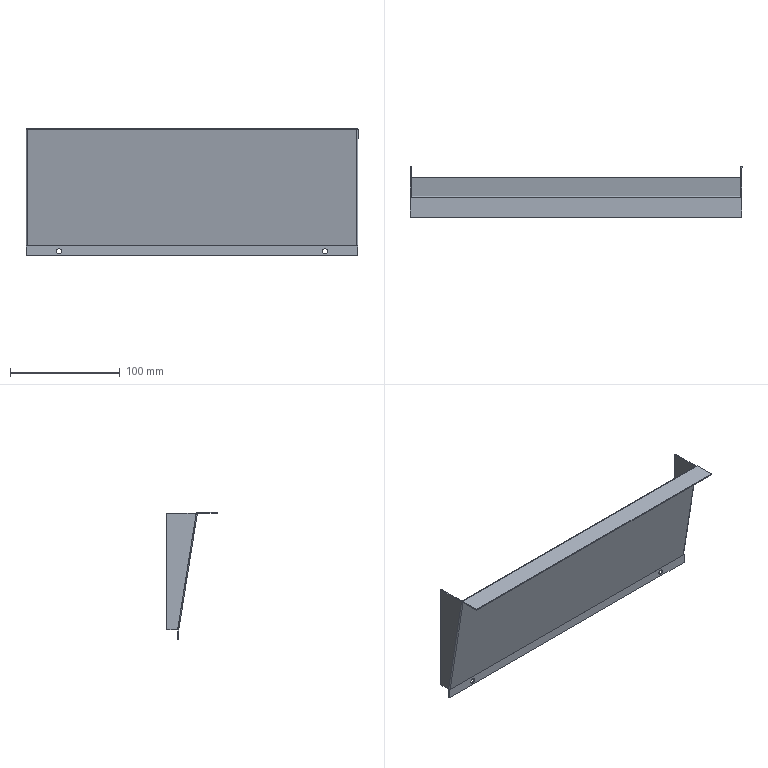Part | SolidWorks | features Cut 1, EdgeFlange 1, FlatPattern 1, MirrorPattern 1, SMBaseFlange 1, SheetMetal 1, UnFold 1 | 1 solid | 46 faces | box 302 x 46 x 116 mm | volume 44658 mm3 | plane 30 | cylinder 12 | spline 4 | commonest cylinder face diameters 0.2 x4 2.2 x4 4.5 x4
STEP:
#1=CARTESIAN_POINT('',(121.,-1.,-2.75));
#2=VERTEX_POINT('',#1);
#3=CARTESIAN_POINT('',(121.,-1.,-7.25));
#4=VERTEX_POINT('',#3);
#5=CARTESIAN_POINT('',(121.,-1.,-5.));
#6=DIRECTION('',(0.,-1.,0.));
#7=DIRECTION('',(0.,0.,-1.));
#8=AXIS2_PLACEMENT_3D('',#5,#6,#7);
#9=CIRCLE('',#8,2.25);
#10=EDGE_CURVE('',#2,#4,#9,.T.);
#11=ORIENTED_EDGE('',*,*,#10,.T.);
#12=CARTESIAN_POINT('',(121.,0.,-7.25));
#13=VERTEX_POINT('',#12);
#14=CARTESIAN_POINT('',(121.,-10.,-7.25));
#15=DIRECTION('',(0.,1.,0.));
#16=VECTOR('',#15,1000.);
#17=LINE('',#14,#16);
#18=EDGE_CURVE('',#4,#13,#17,.T.);
#19=ORIENTED_EDGE('',*,*,#18,.T.);
#20=CARTESIAN_POINT('',(121.,0.,-2.75));
#21=VERTEX_POINT('',#20);
#22=CARTESIAN_POINT('',(121.,0.,-5.));
#23=DIRECTION('',(0.,1.,0.));
#24=DIRECTION('',(0.,0.,1.));
#25=AXIS2_PLACEMENT_3D('',#22,#23,#24);
#26=CIRCLE('',#25,2.25);
#27=EDGE_CURVE('',#13,#21,#26,.T.);
#28=ORIENTED_EDGE('',*,*,#27,.T.);
#29=CARTESIAN_POINT('',(121.,-10.,-2.75));
#30=DIRECTION('',(0.,1.,0.));
#31=VECTOR('',#30,1000.);
#32=LINE('',#29,#31);
#33=EDGE_CURVE('',#2,#21,#32,.T.);
#34=ORIENTED_EDGE('',*,*,#33,.F.);
#35=EDGE_LOOP('',(#11,#19,#28,#34));
#36=FACE_OUTER_BOUND('',#35,.T.);
#37=CARTESIAN_POINT('',(121.,-10.,-5.));
#38=DIRECTION('',(0.,1.,0.));
#39=DIRECTION('',(0.,0.,1.));
#40=AXIS2_PLACEMENT_3D('',#37,#38,#39);
#41=CYLINDRICAL_SURFACE('',#40,2.25);
#42=ADVANCED_FACE('',(#36),#41,.F.);
#43=CARTESIAN_POINT('',(-121.,-1.,-2.75));
#44=VERTEX_POINT('',#43);
#45=CARTESIAN_POINT('',(-121.,-1.,-7.25));
#46=VERTEX_POINT('',#45);
#47=CARTESIAN_POINT('',(-121.,-1.,-5.));
#48=DIRECTION('',(0.,-1.,0.));
#49=DIRECTION('',(0.,0.,-1.));
#50=AXIS2_PLACEMENT_3D('',#47,#48,#49);
#51=CIRCLE('',#50,2.25);
#52=EDGE_CURVE('',#44,#46,#51,.T.);
#53=ORIENTED_EDGE('',*,*,#52,.T.);
#54=CARTESIAN_POINT('',(-121.,0.,-7.25));
#55=VERTEX_POINT('',#54);
#56=CARTESIAN_POINT('',(-121.,-10.,-7.25));
#57=DIRECTION('',(0.,1.,0.));
#58=VECTOR('',#57,1000.);
#59=LINE('',#56,#58);
#60=EDGE_CURVE('',#46,#55,#59,.T.);
#61=ORIENTED_EDGE('',*,*,#60,.T.);
#62=CARTESIAN_POINT('',(-121.,0.,-2.75));
#63=VERTEX_POINT('',#62);
#64=CARTESIAN_POINT('',(-121.,0.,-5.));
#65=DIRECTION('',(0.,1.,0.));
#66=DIRECTION('',(0.,0.,-1.));
#67=AXIS2_PLACEMENT_3D('',#64,#65,#66);
#68=CIRCLE('',#67,2.25);
#69=EDGE_CURVE('',#55,#63,#68,.T.);
#70=ORIENTED_EDGE('',*,*,#69,.T.);
#71=CARTESIAN_POINT('',(-121.,-10.,-2.75));
#72=DIRECTION('',(0.,1.,0.));
#73=VECTOR('',#72,1000.);
#74=LINE('',#71,#73);
#75=EDGE_CURVE('',#44,#63,#74,.T.);
#76=ORIENTED_EDGE('',*,*,#75,.F.);
#77=EDGE_LOOP('',(#53,#61,#70,#76));
#78=FACE_OUTER_BOUND('',#77,.T.);
#79=CARTESIAN_POINT('',(-121.,-10.,-5.));
#80=DIRECTION('',(0.,1.,0.));
#81=DIRECTION('',(0.,0.,1.));
#82=AXIS2_PLACEMENT_3D('',#79,#80,#81);
#83=CYLINDRICAL_SURFACE('',#82,2.25);
#84=ADVANCED_FACE('',(#78),#83,.F.);
#85=CARTESIAN_POINT('',(-149.9,-17.939,106.));
#86=VERTEX_POINT('',#85);
#87=CARTESIAN_POINT('',(-149.9,-17.939,107.));
#88=VERTEX_POINT('',#87);
#89=CARTESIAN_POINT('',(-149.9,-17.939,106.));
#90=DIRECTION('',(0.,0.,1.));
#91=VECTOR('',#90,1000.);
#92=LINE('',#89,#91);
#93=EDGE_CURVE('',#86,#88,#92,.T.);
#94=ORIENTED_EDGE('',*,*,#93,.F.);
#95=CARTESIAN_POINT('',(-151.,-17.939,106.));
#96=VERTEX_POINT('',#95);
#97=CARTESIAN_POINT('',(151.,-17.939,106.));
#98=DIRECTION('',(-1.,0.,0.));
#99=VECTOR('',#98,1000.);
#100=LINE('',#97,#99);
#101=EDGE_CURVE('',#86,#96,#100,.T.);
#102=ORIENTED_EDGE('',*,*,#101,.T.);
#103=CARTESIAN_POINT('',(-151.,-17.939,107.));
#104=VERTEX_POINT('',#103);
#105=CARTESIAN_POINT('',(-151.,-17.939,107.));
#106=DIRECTION('',(0.,0.,-1.));
#107=VECTOR('',#106,1000.);
#108=LINE('',#105,#107);
#109=EDGE_CURVE('',#104,#96,#108,.T.);
#110=ORIENTED_EDGE('',*,*,#109,.F.);
#111=CARTESIAN_POINT('',(151.,-17.939,107.));
#112=DIRECTION('',(-1.,0.,0.));
#113=VECTOR('',#112,1000.);
#114=LINE('',#111,#113);
#115=EDGE_CURVE('',#88,#104,#114,.T.);
#116=ORIENTED_EDGE('',*,*,#115,.F.);
#117=EDGE_LOOP('',(#94,#102,#110,#116));
#118=FACE_OUTER_BOUND('',#117,.T.);
#119=CARTESIAN_POINT('',(0.,-17.939,0.));
#120=DIRECTION('',(0.,-1.,0.));
#121=DIRECTION('',(0.,0.,-1.));
#122=AXIS2_PLACEMENT_3D('',#119,#120,#121);
#123=PLANE('',#122);
#124=ADVANCED_FACE('',(#118),#123,.F.);
#125=CARTESIAN_POINT('',(149.9,-17.939,106.));
#126=VERTEX_POINT('',#125);
#127=CARTESIAN_POINT('',(151.,-17.939,106.));
#128=DIRECTION('',(-1.,0.,0.));
#129=VECTOR('',#128,1000.);
#130=LINE('',#127,#129);
#131=EDGE_CURVE('',#126,#86,#130,.T.);
#132=ORIENTED_EDGE('',*,*,#131,.T.);
#133=CARTESIAN_POINT('',(-149.9,-17.84,105.916));
#134=VERTEX_POINT('',#133);
#135=CARTESIAN_POINT('',(-149.9,-17.939,105.9));
#136=DIRECTION('',(-1.,0.,0.));
#137=DIRECTION('',(0.,0.,1.));
#138=AXIS2_PLACEMENT_3D('',#135,#136,#137);
#139=CIRCLE('',#138,0.1);
#140=EDGE_CURVE('',#86,#134,#139,.T.);
#141=ORIENTED_EDGE('',*,*,#140,.T.);
#142=CARTESIAN_POINT('',(149.9,-17.84,105.916));
#143=VERTEX_POINT('',#142);
#144=CARTESIAN_POINT('',(151.,-17.84,105.916));
#145=DIRECTION('',(-1.,0.,0.));
#146=VECTOR('',#145,1000.);
#147=LINE('',#144,#146);
#148=EDGE_CURVE('',#143,#134,#147,.T.);
#149=ORIENTED_EDGE('',*,*,#148,.F.);
#150=CARTESIAN_POINT('',(149.9,-17.939,105.9));
#151=DIRECTION('',(1.,0.,0.));
#152=DIRECTION('',(0.,0.,-1.));
#153=AXIS2_PLACEMENT_3D('',#150,#151,#152);
#154=CIRCLE('',#153,0.1);
#155=EDGE_CURVE('',#143,#126,#154,.T.);
#156=ORIENTED_EDGE('',*,*,#155,.T.);
#157=EDGE_LOOP('',(#132,#141,#149,#156));
#158=FACE_OUTER_BOUND('',#157,.T.);
#159=CARTESIAN_POINT('',(151.,-17.939,105.9));
#160=DIRECTION('',(-1.,0.,0.));
#161=DIRECTION('',(0.,0.,1.));
#162=AXIS2_PLACEMENT_3D('',#159,#160,#161);
#163=CYLINDRICAL_SURFACE('',#162,0.1);
#164=ADVANCED_FACE('',(#158),#163,.F.);
#165=CARTESIAN_POINT('',(-149.9,0.,-0.08684));
#166=VERTEX_POINT('',#165);
#167=CARTESIAN_POINT('',(-149.9,-1.,-0.08684));
#168=VERTEX_POINT('',#167);
#169=CARTESIAN_POINT('',(-149.9,0.,-0.08684));
#170=DIRECTION('',(0.,-1.,0.));
#171=VECTOR('',#170,1000.);
#172=LINE('',#169,#171);
#173=EDGE_CURVE('',#166,#168,#172,.T.);
#174=ORIENTED_EDGE('',*,*,#173,.F.);
#175=CARTESIAN_POINT('',(-151.,0.,-0.08684));
#176=VERTEX_POINT('',#175);
#177=CARTESIAN_POINT('',(151.,0.,-0.08684));
#178=DIRECTION('',(-1.,0.,0.));
#179=VECTOR('',#178,1000.);
#180=LINE('',#177,#179);
#181=EDGE_CURVE('',#166,#176,#180,.T.);
#182=ORIENTED_EDGE('',*,*,#181,.T.);
#183=CARTESIAN_POINT('',(-151.,-1.,-0.08684));
#184=VERTEX_POINT('',#183);
#185=CARTESIAN_POINT('',(-151.,-1.,-0.08684));
#186=DIRECTION('',(0.,1.,0.));
#187=VECTOR('',#186,1000.);
#188=LINE('',#185,#187);
#189=EDGE_CURVE('',#184,#176,#188,.T.);
#190=ORIENTED_EDGE('',*,*,#189,.F.);
#191=CARTESIAN_POINT('',(151.,-1.,-0.08684));
#192=DIRECTION('',(-1.,0.,0.));
#193=VECTOR('',#192,1000.);
#194=LINE('',#191,#193);
#195=EDGE_CURVE('',#168,#184,#194,.T.);
#196=ORIENTED_EDGE('',*,*,#195,.F.);
#197=EDGE_LOOP('',(#174,#182,#190,#196));
#198=FACE_OUTER_BOUND('',#197,.T.);
#199=CARTESIAN_POINT('',(0.,0.,-0.08684));
#200=DIRECTION('',(0.,0.,-1.));
#201=DIRECTION('',(-1.,0.,0.));
#202=AXIS2_PLACEMENT_3D('',#199,#200,#201);
#203=PLANE('',#202);
#204=ADVANCED_FACE('',(#198),#203,.F.);
#205=CARTESIAN_POINT('',(149.9,-1.001,-0.07115));
#206=VERTEX_POINT('',#205);
#207=CARTESIAN_POINT('',(-149.9,-1.001,-0.07115));
#208=VERTEX_POINT('',#207);
#209=CARTESIAN_POINT('',(151.,-1.001,-0.07115));
#210=DIRECTION('',(-1.,0.,0.));
#211=VECTOR('',#210,1000.);
#212=LINE('',#209,#211);
#213=EDGE_CURVE('',#206,#208,#212,.T.);
#214=ORIENTED_EDGE('',*,*,#213,.T.);
#215=CARTESIAN_POINT('',(-149.9,-1.1,-0.08684));
#216=DIRECTION('',(-1.,0.,0.));
#217=DIRECTION('',(0.,0.,1.));
#218=AXIS2_PLACEMENT_3D('',#215,#216,#217);
#219=CIRCLE('',#218,0.1);
#220=EDGE_CURVE('',#208,#168,#219,.T.);
#221=ORIENTED_EDGE('',*,*,#220,.T.);
#222=CARTESIAN_POINT('',(149.9,-1.,-0.08684));
#223=VERTEX_POINT('',#222);
#224=CARTESIAN_POINT('',(151.,-1.,-0.08684));
#225=DIRECTION('',(-1.,0.,0.));
#226=VECTOR('',#225,1000.);
#227=LINE('',#224,#226);
#228=EDGE_CURVE('',#223,#168,#227,.T.);
#229=ORIENTED_EDGE('',*,*,#228,.F.);
#230=CARTESIAN_POINT('',(149.9,-1.1,-0.08684));
#231=DIRECTION('',(1.,0.,0.));
#232=DIRECTION('',(0.,0.,-1.));
#233=AXIS2_PLACEMENT_3D('',#230,#231,#232);
#234=CIRCLE('',#233,0.1);
#235=EDGE_CURVE('',#223,#206,#234,.T.);
#236=ORIENTED_EDGE('',*,*,#235,.T.);
#237=EDGE_LOOP('',(#214,#221,#229,#236));
#238=FACE_OUTER_BOUND('',#237,.T.);
#239=CARTESIAN_POINT('',(151.,-1.1,-0.08684));
#240=DIRECTION('',(-1.,0.,0.));
#241=DIRECTION('',(0.,0.,1.));
#242=AXIS2_PLACEMENT_3D('',#239,#240,#241);
#243=CYLINDRICAL_SURFACE('',#242,0.1);
#244=ADVANCED_FACE('',(#238),#243,.F.);
#245=CARTESIAN_POINT('',(-149.9,-0.01363,0.08576));
#246=VERTEX_POINT('',#245);
#247=CARTESIAN_POINT('',(-149.9,-1.1,-0.08684));
#248=DIRECTION('',(-1.,0.,0.));
#249=DIRECTION('',(0.,0.,1.));
#250=AXIS2_PLACEMENT_3D('',#247,#248,#249);
#251=CIRCLE('',#250,1.1);
#252=EDGE_CURVE('',#246,#166,#251,.T.);
#253=ORIENTED_EDGE('',*,*,#252,.T.);
#254=ORIENTED_EDGE('',*,*,#173,.T.);
#255=ORIENTED_EDGE('',*,*,#220,.F.);
#256=CARTESIAN_POINT('',(-149.9,-0.01363,0.08576));
#257=DIRECTION('',(0.,-0.9876,-0.1569));
#258=VECTOR('',#257,1000.);
#259=LINE('',#256,#258);
#260=EDGE_CURVE('',#246,#208,#259,.T.);
#261=ORIENTED_EDGE('',*,*,#260,.F.);
#262=EDGE_LOOP('',(#253,#254,#255,#261));
#263=FACE_OUTER_BOUND('',#262,.T.);
#264=CARTESIAN_POINT('',(-149.9,-1.1,-0.08684));
#265=DIRECTION('',(-1.,0.,0.));
#266=DIRECTION('',(0.,0.,1.));
#267=AXIS2_PLACEMENT_3D('',#264,#265,#266);
#268=PLANE('',#267);
#269=ADVANCED_FACE('',(#263),#268,.T.);
#270=ORIENTED_EDGE('',*,*,#148,.T.);
#271=CARTESIAN_POINT('',(-149.9,-17.84,105.916));
#272=DIRECTION('',(0.,0.1569,-0.9876));
#273=VECTOR('',#272,1000.);
#274=LINE('',#271,#273);
#275=EDGE_CURVE('',#134,#208,#274,.T.);
#276=ORIENTED_EDGE('',*,*,#275,.T.);
#277=ORIENTED_EDGE('',*,*,#213,.F.);
#278=CARTESIAN_POINT('',(149.9,-0.9987,-0.08684));
#279=DIRECTION('',(0.,-0.1569,0.9876));
#280=VECTOR('',#279,1000.);
#281=LINE('',#278,#280);
#282=EDGE_CURVE('',#206,#143,#281,.T.);
#283=ORIENTED_EDGE('',*,*,#282,.T.);
#284=EDGE_LOOP('',(#270,#276,#277,#283));
#285=FACE_OUTER_BOUND('',#284,.T.);
#286=CARTESIAN_POINT('',(151.,-0.9876,-0.1569));
#287=DIRECTION('',(0.,-0.9876,-0.1569));
#288=DIRECTION('',(0.,0.1569,-0.9876));
#289=AXIS2_PLACEMENT_3D('',#286,#287,#288);
#290=PLANE('',#289);
#291=ADVANCED_FACE('',(#285),#290,.T.);
#292=CARTESIAN_POINT('',(-149.9,-16.853,106.073));
#293=VERTEX_POINT('',#292);
#294=CARTESIAN_POINT('',(-149.9,-16.853,106.073));
#295=DIRECTION('',(0.,0.1569,-0.9876));
#296=VECTOR('',#295,1000.);
#297=LINE('',#294,#296);
#298=EDGE_CURVE('',#293,#246,#297,.T.);
#299=ORIENTED_EDGE('',*,*,#298,.F.);
#300=CARTESIAN_POINT('',(149.9,-16.853,106.073));
#301=VERTEX_POINT('',#300);
#302=CARTESIAN_POINT('',(151.,-16.853,106.073));
#303=DIRECTION('',(-1.,0.,0.));
#304=VECTOR('',#303,1000.);
#305=LINE('',#302,#304);
#306=EDGE_CURVE('',#301,#293,#305,.T.);
#307=ORIENTED_EDGE('',*,*,#306,.F.);
#308=CARTESIAN_POINT('',(149.9,-0.01363,0.08576));
#309=VERTEX_POINT('',#308);
#310=CARTESIAN_POINT('',(149.9,-0.01113,0.07007));
#311=DIRECTION('',(0.,-0.1569,0.9876));
#312=VECTOR('',#311,1000.);
#313=LINE('',#310,#312);
#314=EDGE_CURVE('',#309,#301,#313,.T.);
#315=ORIENTED_EDGE('',*,*,#314,.F.);
#316=CARTESIAN_POINT('',(151.,-0.01363,0.08576));
#317=DIRECTION('',(-1.,0.,0.));
#318=VECTOR('',#317,1000.);
#319=LINE('',#316,#318);
#320=EDGE_CURVE('',#309,#246,#319,.T.);
#321=ORIENTED_EDGE('',*,*,#320,.T.);
#322=EDGE_LOOP('',(#299,#307,#315,#321));
#323=FACE_OUTER_BOUND('',#322,.T.);
#324=CARTESIAN_POINT('',(151.,0.,0.));
#325=DIRECTION('',(0.,-0.9876,-0.1569));
#326=DIRECTION('',(0.,0.1569,-0.9876));
#327=AXIS2_PLACEMENT_3D('',#324,#325,#326);
#328=PLANE('',#327);
#329=ADVANCED_FACE('',(#323),#328,.F.);
#330=CARTESIAN_POINT('',(149.9,0.,-0.08684));
#331=VERTEX_POINT('',#330);
#332=CARTESIAN_POINT('',(149.9,-1.,-0.08684));
#333=DIRECTION('',(0.,1.,0.));
#334=VECTOR('',#333,1000.);
#335=LINE('',#332,#334);
#336=EDGE_CURVE('',#223,#331,#335,.T.);
#337=ORIENTED_EDGE('',*,*,#336,.F.);
#338=CARTESIAN_POINT('',(151.,-1.,-0.08684));
#339=VERTEX_POINT('',#338);
#340=CARTESIAN_POINT('',(151.,-1.,-0.08684));
#341=DIRECTION('',(-1.,0.,0.));
#342=VECTOR('',#341,1000.);
#343=LINE('',#340,#342);
#344=EDGE_CURVE('',#339,#223,#343,.T.);
#345=ORIENTED_EDGE('',*,*,#344,.F.);
#346=CARTESIAN_POINT('',(151.,0.,-0.08684));
#347=VERTEX_POINT('',#346);
#348=CARTESIAN_POINT('',(151.,0.,-0.08684));
#349=DIRECTION('',(0.,-1.,0.));
#350=VECTOR('',#349,1000.);
#351=LINE('',#348,#350);
#352=EDGE_CURVE('',#347,#339,#351,.T.);
#353=ORIENTED_EDGE('',*,*,#352,.F.);
#354=CARTESIAN_POINT('',(151.,0.,-0.08684));
#355=DIRECTION('',(-1.,0.,0.));
#356=VECTOR('',#355,1000.);
#357=LINE('',#354,#356);
#358=EDGE_CURVE('',#347,#331,#357,.T.);
#359=ORIENTED_EDGE('',*,*,#358,.T.);
#360=EDGE_LOOP('',(#337,#345,#353,#359));
#361=FACE_OUTER_BOUND('',#360,.T.);
#362=CARTESIAN_POINT('',(0.,0.,-0.08684));
#363=DIRECTION('',(0.,0.,1.));
#364=DIRECTION('',(1.,0.,0.));
#365=AXIS2_PLACEMENT_3D('',#362,#363,#364);
#366=PLANE('',#365);
#367=ADVANCED_FACE('',(#361),#366,.T.);
#368=CARTESIAN_POINT('',(149.9,-17.939,107.));
#369=VERTEX_POINT('',#368);
#370=CARTESIAN_POINT('',(149.9,-17.939,107.));
#371=DIRECTION('',(0.,0.,-1.));
#372=VECTOR('',#371,1000.);
#373=LINE('',#370,#372);
#374=EDGE_CURVE('',#369,#126,#373,.T.);
#375=ORIENTED_EDGE('',*,*,#374,.F.);
#376=CARTESIAN_POINT('',(151.,-17.939,107.));
#377=VERTEX_POINT('',#376);
#378=CARTESIAN_POINT('',(151.,-17.939,107.));
#379=DIRECTION('',(-1.,0.,0.));
#380=VECTOR('',#379,1000.);
#381=LINE('',#378,#380);
#382=EDGE_CURVE('',#377,#369,#381,.T.);
#383=ORIENTED_EDGE('',*,*,#382,.F.);
#384=CARTESIAN_POINT('',(151.,-17.939,106.));
#385=VERTEX_POINT('',#384);
#386=CARTESIAN_POINT('',(151.,-17.939,106.));
#387=DIRECTION('',(0.,0.,1.));
#388=VECTOR('',#387,1000.);
#389=LINE('',#386,#388);
#390=EDGE_CURVE('',#385,#377,#389,.T.);
#391=ORIENTED_EDGE('',*,*,#390,.F.);
#392=CARTESIAN_POINT('',(151.,-17.939,106.));
#393=DIRECTION('',(-1.,0.,0.));
#394=VECTOR('',#393,1000.);
#395=LINE('',#392,#394);
#396=EDGE_CURVE('',#385,#126,#395,.T.);
#397=ORIENTED_EDGE('',*,*,#396,.T.);
#398=EDGE_LOOP('',(#375,#383,#391,#397));
#399=FACE_OUTER_BOUND('',#398,.T.);
#400=CARTESIAN_POINT('',(0.,-17.939,0.));
#401=DIRECTION('',(0.,1.,0.));
#402=DIRECTION('',(0.,0.,1.));
#403=AXIS2_PLACEMENT_3D('',#400,#401,#402);
#404=PLANE('',#403);
#405=ADVANCED_FACE('',(#399),#404,.T.);
#406=ORIENTED_EDGE('',*,*,#140,.F.);
#407=ORIENTED_EDGE('',*,*,#93,.T.);
#408=CARTESIAN_POINT('',(-149.9,-17.939,105.9));
#409=DIRECTION('',(-1.,0.,0.));
#410=DIRECTION('',(0.,0.,1.));
#411=AXIS2_PLACEMENT_3D('',#408,#409,#410);
#412=CIRCLE('',#411,1.1);
#413=EDGE_CURVE('',#88,#293,#412,.T.);
#414=ORIENTED_EDGE('',*,*,#413,.T.);
#415=CARTESIAN_POINT('',(-149.9,-16.853,106.073));
#416=DIRECTION('',(0.,-0.9876,-0.1569));
#417=VECTOR('',#416,1000.);
#418=LINE('',#415,#417);
#419=EDGE_CURVE('',#293,#134,#418,.T.);
#420=ORIENTED_EDGE('',*,*,#419,.T.);
#421=EDGE_LOOP('',(#406,#407,#414,#420));
#422=FACE_OUTER_BOUND('',#421,.T.);
#423=CARTESIAN_POINT('',(-149.9,-17.939,105.9));
#424=DIRECTION('',(-1.,0.,0.));
#425=DIRECTION('',(0.,0.,1.));
#426=AXIS2_PLACEMENT_3D('',#423,#424,#425);
#427=PLANE('',#426);
#428=ADVANCED_FACE('',(#422),#427,.T.);
#429=CARTESIAN_POINT('',(149.9,-17.939,105.9));
#430=DIRECTION('',(1.,0.,0.));
#431=DIRECTION('',(0.,0.,-1.));
#432=AXIS2_PLACEMENT_3D('',#429,#430,#431);
#433=CIRCLE('',#432,1.1);
#434=EDGE_CURVE('',#301,#369,#433,.T.);
#435=ORIENTED_EDGE('',*,*,#434,.T.);
#436=ORIENTED_EDGE('',*,*,#374,.T.);
#437=ORIENTED_EDGE('',*,*,#155,.F.);
#438=CARTESIAN_POINT('',(149.9,-16.853,106.073));
#439=DIRECTION('',(0.,-0.9876,-0.1569));
#440=VECTOR('',#439,1000.);
#441=LINE('',#438,#440);
#442=EDGE_CURVE('',#301,#143,#441,.T.);
#443=ORIENTED_EDGE('',*,*,#442,.F.);
#444=EDGE_LOOP('',(#435,#436,#437,#443));
#445=FACE_OUTER_BOUND('',#444,.T.);
#446=CARTESIAN_POINT('',(149.9,-17.939,105.9));
#447=DIRECTION('',(1.,0.,0.));
#448=DIRECTION('',(0.,0.,-1.));
#449=AXIS2_PLACEMENT_3D('',#446,#447,#448);
#450=PLANE('',#449);
#451=ADVANCED_FACE('',(#445),#450,.T.);
#452=CARTESIAN_POINT('',(151.,0.,-9.));
#453=VERTEX_POINT('',#452);
#454=CARTESIAN_POINT('',(151.,0.,0.));
#455=DIRECTION('',(0.,0.,1.));
#456=VECTOR('',#455,1000.);
#457=LINE('',#454,#456);
#458=EDGE_CURVE('',#453,#347,#457,.T.);
#459=ORIENTED_EDGE('',*,*,#458,.T.);
#460=ORIENTED_EDGE('',*,*,#352,.T.);
#461=CARTESIAN_POINT('',(151.,-1.,-9.));
#462=VERTEX_POINT('',#461);
#463=CARTESIAN_POINT('',(151.,-1.,0.));
#464=DIRECTION('',(0.,0.,1.));
#465=VECTOR('',#464,1000.);
#466=LINE('',#463,#465);
#467=EDGE_CURVE('',#462,#339,#466,.T.);
#468=ORIENTED_EDGE('',*,*,#467,.F.);
#469=CARTESIAN_POINT('',(151.,0.,-9.));
#470=DIRECTION('',(0.,-1.,0.));
#471=VECTOR('',#470,1000.);
#472=LINE('',#469,#471);
#473=EDGE_CURVE('',#453,#462,#472,.T.);
#474=ORIENTED_EDGE('',*,*,#473,.F.);
#475=EDGE_LOOP('',(#459,#460,#468,#474));
#476=FACE_OUTER_BOUND('',#475,.T.);
#477=CARTESIAN_POINT('',(151.,-1.001,-0.07115));
#478=DIRECTION('',(1.,0.,0.));
#479=DIRECTION('',(0.,0.,-1.));
#480=AXIS2_PLACEMENT_3D('',#477,#478,#479);
#481=PLANE('',#480);
#482=ADVANCED_FACE('',(#476),#481,.T.);
#483=CARTESIAN_POINT('',(-151.,-36.,107.));
#484=VERTEX_POINT('',#483);
#485=CARTESIAN_POINT('',(-151.,-17.,107.));
#486=DIRECTION('',(0.,-1.,0.));
#487=VECTOR('',#486,1000.);
#488=LINE('',#485,#487);
#489=EDGE_CURVE('',#104,#484,#488,.T.);
#490=ORIENTED_EDGE('',*,*,#489,.F.);
#491=ORIENTED_EDGE('',*,*,#109,.T.);
#492=CARTESIAN_POINT('',(-151.,-36.,106.));
#493=VERTEX_POINT('',#492);
#494=CARTESIAN_POINT('',(-151.,-17.,106.));
#495=DIRECTION('',(0.,-1.,0.));
#496=VECTOR('',#495,1000.);
#497=LINE('',#494,#496);
#498=EDGE_CURVE('',#96,#493,#497,.T.);
#499=ORIENTED_EDGE('',*,*,#498,.T.);
#500=CARTESIAN_POINT('',(-151.,-36.,106.));
#501=DIRECTION('',(0.,0.,1.));
#502=VECTOR('',#501,1000.);
#503=LINE('',#500,#502);
#504=EDGE_CURVE('',#493,#484,#503,.T.);
#505=ORIENTED_EDGE('',*,*,#504,.T.);
#506=EDGE_LOOP('',(#490,#491,#499,#505));
#507=FACE_OUTER_BOUND('',#506,.T.);
#508=CARTESIAN_POINT('',(-151.,-17.84,105.916));
#509=DIRECTION('',(-1.,0.,0.));
#510=DIRECTION('',(0.,0.,1.));
#511=AXIS2_PLACEMENT_3D('',#508,#509,#510);
#512=PLANE('',#511);
#513=ADVANCED_FACE('',(#507),#512,.T.);
#514=ORIENTED_EDGE('',*,*,#489,.T.);
#515=CARTESIAN_POINT('',(151.,-36.,107.));
#516=VERTEX_POINT('',#515);
#517=CARTESIAN_POINT('',(151.,-36.,107.));
#518=DIRECTION('',(-1.,0.,0.));
#519=VECTOR('',#518,1000.);
#520=LINE('',#517,#519);
#521=EDGE_CURVE('',#516,#484,#520,.T.);
#522=ORIENTED_EDGE('',*,*,#521,.F.);
#523=CARTESIAN_POINT('',(151.,-17.,107.));
#524=DIRECTION('',(0.,-1.,0.));
#525=VECTOR('',#524,1000.);
#526=LINE('',#523,#525);
#527=EDGE_CURVE('',#377,#516,#526,.T.);
#528=ORIENTED_EDGE('',*,*,#527,.F.);
#529=ORIENTED_EDGE('',*,*,#382,.T.);
#530=CARTESIAN_POINT('',(151.,-17.939,107.));
#531=DIRECTION('',(-1.,0.,0.));
#532=VECTOR('',#531,1000.);
#533=LINE('',#530,#532);
#534=EDGE_CURVE('',#369,#88,#533,.T.);
#535=ORIENTED_EDGE('',*,*,#534,.T.);
#536=ORIENTED_EDGE('',*,*,#115,.T.);
#537=EDGE_LOOP('',(#514,#522,#528,#529,#535,#536));
#538=FACE_OUTER_BOUND('',#537,.T.);
#539=CARTESIAN_POINT('',(151.,-17.,107.));
#540=DIRECTION('',(0.,0.,-1.));
#541=DIRECTION('',(-1.,0.,0.));
#542=AXIS2_PLACEMENT_3D('',#539,#540,#541);
#543=PLANE('',#542);
#544=ADVANCED_FACE('',(#538),#543,.F.);
#545=ORIENTED_EDGE('',*,*,#504,.F.);
#546=CARTESIAN_POINT('',(151.,-36.,106.));
#547=VERTEX_POINT('',#546);
#548=CARTESIAN_POINT('',(151.,-36.,106.));
#549=DIRECTION('',(-1.,0.,0.));
#550=VECTOR('',#549,1000.);
#551=LINE('',#548,#550);
#552=EDGE_CURVE('',#547,#493,#551,.T.);
#553=ORIENTED_EDGE('',*,*,#552,.F.);
#554=CARTESIAN_POINT('',(151.,-36.,106.));
#555=DIRECTION('',(0.,0.,1.));
#556=VECTOR('',#555,1000.);
#557=LINE('',#554,#556);
#558=EDGE_CURVE('',#547,#516,#557,.T.);
#559=ORIENTED_EDGE('',*,*,#558,.T.);
#560=ORIENTED_EDGE('',*,*,#521,.T.);
#561=EDGE_LOOP('',(#545,#553,#559,#560));
#562=FACE_OUTER_BOUND('',#561,.T.);
#563=CARTESIAN_POINT('',(151.,-36.,106.));
#564=DIRECTION('',(0.,-1.,0.));
#565=DIRECTION('',(0.,0.,-1.));
#566=AXIS2_PLACEMENT_3D('',#563,#564,#565);
#567=PLANE('',#566);
#568=ADVANCED_FACE('',(#562),#567,.T.);
#569=ORIENTED_EDGE('',*,*,#498,.F.);
#570=ORIENTED_EDGE('',*,*,#101,.F.);
#571=ORIENTED_EDGE('',*,*,#131,.F.);
#572=ORIENTED_EDGE('',*,*,#396,.F.);
#573=CARTESIAN_POINT('',(151.,-17.,106.));
#574=DIRECTION('',(0.,-1.,0.));
#575=VECTOR('',#574,1000.);
#576=LINE('',#573,#575);
#577=EDGE_CURVE('',#385,#547,#576,.T.);
#578=ORIENTED_EDGE('',*,*,#577,.T.);
#579=ORIENTED_EDGE('',*,*,#552,.T.);
#580=EDGE_LOOP('',(#569,#570,#571,#572,#578,#579));
#581=FACE_OUTER_BOUND('',#580,.T.);
#582=CARTESIAN_POINT('',(151.,-17.,106.));
#583=DIRECTION('',(0.,0.,-1.));
#584=DIRECTION('',(-1.,0.,0.));
#585=AXIS2_PLACEMENT_3D('',#582,#583,#584);
#586=PLANE('',#585);
#587=ADVANCED_FACE('',(#581),#586,.T.);
#588=ORIENTED_EDGE('',*,*,#235,.F.);
#589=ORIENTED_EDGE('',*,*,#336,.T.);
#590=CARTESIAN_POINT('',(149.9,-1.1,-0.08684));
#591=DIRECTION('',(1.,0.,0.));
#592=DIRECTION('',(0.,0.,-1.));
#593=AXIS2_PLACEMENT_3D('',#590,#591,#592);
#594=CIRCLE('',#593,1.1);
#595=EDGE_CURVE('',#331,#309,#594,.T.);
#596=ORIENTED_EDGE('',*,*,#595,.T.);
#597=CARTESIAN_POINT('',(149.9,-0.01363,0.08576));
#598=DIRECTION('',(0.,-0.9876,-0.1569));
#599=VECTOR('',#598,1000.);
#600=LINE('',#597,#599);
#601=EDGE_CURVE('',#309,#206,#600,.T.);
#602=ORIENTED_EDGE('',*,*,#601,.T.);
#603=EDGE_LOOP('',(#588,#589,#596,#602));
#604=FACE_OUTER_BOUND('',#603,.T.);
#605=CARTESIAN_POINT('',(149.9,-1.1,-0.08684));
#606=DIRECTION('',(1.,0.,0.));
#607=DIRECTION('',(0.,0.,-1.));
#608=AXIS2_PLACEMENT_3D('',#605,#606,#607);
#609=PLANE('',#608);
#610=ADVANCED_FACE('',(#604),#609,.T.);
#611=ORIENTED_EDGE('',*,*,#10,.F.);
#612=CARTESIAN_POINT('',(121.,-1.,-5.));
#613=DIRECTION('',(0.,-1.,0.));
#614=DIRECTION('',(0.,0.,-1.));
#615=AXIS2_PLACEMENT_3D('',#612,#613,#614);
#616=CIRCLE('',#615,2.25);
#617=EDGE_CURVE('',#4,#2,#616,.T.);
#618=ORIENTED_EDGE('',*,*,#617,.F.);
#619=EDGE_LOOP('',(#611,#618));
#620=FACE_BOUND('',#619,.T.);
#621=ORIENTED_EDGE('',*,*,#52,.F.);
#622=CARTESIAN_POINT('',(-121.,-1.,-5.));
#623=DIRECTION('',(0.,-1.,0.));
#624=DIRECTION('',(0.,0.,-1.));
#625=AXIS2_PLACEMENT_3D('',#622,#623,#624);
#626=CIRCLE('',#625,2.25);
#627=EDGE_CURVE('',#46,#44,#626,.T.);
#628=ORIENTED_EDGE('',*,*,#627,.F.);
#629=EDGE_LOOP('',(#621,#628));
#630=FACE_BOUND('',#629,.T.);
#631=CARTESIAN_POINT('',(-151.,-1.,-9.));
#632=VERTEX_POINT('',#631);
#633=CARTESIAN_POINT('',(-151.,-1.,0.));
#634=DIRECTION('',(0.,0.,1.));
#635=VECTOR('',#634,1000.);
#636=LINE('',#633,#635);
#637=EDGE_CURVE('',#632,#184,#636,.T.);
#638=ORIENTED_EDGE('',*,*,#637,.F.);
#639=CARTESIAN_POINT('',(151.,-1.,-9.));
#640=DIRECTION('',(-1.,0.,0.));
#641=VECTOR('',#640,1000.);
#642=LINE('',#639,#641);
#643=EDGE_CURVE('',#462,#632,#642,.T.);
#644=ORIENTED_EDGE('',*,*,#643,.F.);
#645=ORIENTED_EDGE('',*,*,#467,.T.);
#646=ORIENTED_EDGE('',*,*,#344,.T.);
#647=ORIENTED_EDGE('',*,*,#228,.T.);
#648=ORIENTED_EDGE('',*,*,#195,.T.);
#649=EDGE_LOOP('',(#638,#644,#645,#646,#647,#648));
#650=FACE_OUTER_BOUND('',#649,.T.);
#651=CARTESIAN_POINT('',(151.,-1.,0.));
#652=DIRECTION('',(0.,-1.,0.));
#653=DIRECTION('',(0.,0.,-1.));
#654=AXIS2_PLACEMENT_3D('',#651,#652,#653);
#655=PLANE('',#654);
#656=ADVANCED_FACE('',(#620,#630,#650),#655,.T.);
#657=CARTESIAN_POINT('',(-151.,0.,-9.));
#658=VERTEX_POINT('',#657);
#659=CARTESIAN_POINT('',(-151.,0.,-9.));
#660=DIRECTION('',(0.,-1.,0.));
#661=VECTOR('',#660,1000.);
#662=LINE('',#659,#661);
#663=EDGE_CURVE('',#658,#632,#662,.T.);
#664=ORIENTED_EDGE('',*,*,#663,.F.);
#665=CARTESIAN_POINT('',(151.,0.,-9.));
#666=DIRECTION('',(-1.,0.,0.));
#667=VECTOR('',#666,1000.);
#668=LINE('',#665,#667);
#669=EDGE_CURVE('',#453,#658,#668,.T.);
#670=ORIENTED_EDGE('',*,*,#669,.F.);
#671=ORIENTED_EDGE('',*,*,#473,.T.);
#672=ORIENTED_EDGE('',*,*,#643,.T.);
#673=EDGE_LOOP('',(#664,#670,#671,#672));
#674=FACE_OUTER_BOUND('',#673,.T.);
#675=CARTESIAN_POINT('',(151.,0.,-9.));
#676=DIRECTION('',(0.,0.,-1.));
#677=DIRECTION('',(-1.,0.,0.));
#678=AXIS2_PLACEMENT_3D('',#675,#676,#677);
#679=PLANE('',#678);
#680=ADVANCED_FACE('',(#674),#679,.T.);
#681=CARTESIAN_POINT('',(121.,0.,-5.));
#682=DIRECTION('',(0.,1.,0.));
#683=DIRECTION('',(0.,0.,1.));
#684=AXIS2_PLACEMENT_3D('',#681,#682,#683);
#685=CIRCLE('',#684,2.25);
#686=EDGE_CURVE('',#21,#13,#685,.T.);
#687=ORIENTED_EDGE('',*,*,#686,.F.);
#688=ORIENTED_EDGE('',*,*,#27,.F.);
#689=EDGE_LOOP('',(#687,#688));
#690=FACE_BOUND('',#689,.T.);
#691=CARTESIAN_POINT('',(-121.,0.,-5.));
#692=DIRECTION('',(0.,1.,0.));
#693=DIRECTION('',(0.,0.,-1.));
#694=AXIS2_PLACEMENT_3D('',#691,#692,#693);
#695=CIRCLE('',#694,2.25);
#696=EDGE_CURVE('',#63,#55,#695,.T.);
#697=ORIENTED_EDGE('',*,*,#696,.F.);
#698=ORIENTED_EDGE('',*,*,#69,.F.);
#699=EDGE_LOOP('',(#697,#698));
#700=FACE_BOUND('',#699,.T.);
#701=CARTESIAN_POINT('',(-151.,0.,0.));
#702=DIRECTION('',(0.,0.,1.));
#703=VECTOR('',#702,1000.);
#704=LINE('',#701,#703);
#705=EDGE_CURVE('',#658,#176,#704,.T.);
#706=ORIENTED_EDGE('',*,*,#705,.T.);
#707=ORIENTED_EDGE('',*,*,#181,.F.);
#708=CARTESIAN_POINT('',(151.,0.,-0.08684));
#709=DIRECTION('',(-1.,0.,0.));
#710=VECTOR('',#709,1000.);
#711=LINE('',#708,#710);
#712=EDGE_CURVE('',#331,#166,#711,.T.);
#713=ORIENTED_EDGE('',*,*,#712,.F.);
#714=ORIENTED_EDGE('',*,*,#358,.F.);
#715=ORIENTED_EDGE('',*,*,#458,.F.);
#716=ORIENTED_EDGE('',*,*,#669,.T.);
#717=EDGE_LOOP('',(#706,#707,#713,#714,#715,#716));
#718=FACE_OUTER_BOUND('',#717,.T.);
#719=CARTESIAN_POINT('',(151.,0.,0.));
#720=DIRECTION('',(0.,-1.,0.));
#721=DIRECTION('',(0.,0.,-1.));
#722=AXIS2_PLACEMENT_3D('',#719,#720,#721);
#723=PLANE('',#722);
#724=ADVANCED_FACE('',(#690,#700,#718),#723,.F.);
#725=ORIENTED_EDGE('',*,*,#252,.F.);
#726=ORIENTED_EDGE('',*,*,#320,.F.);
#727=ORIENTED_EDGE('',*,*,#595,.F.);
#728=ORIENTED_EDGE('',*,*,#712,.T.);
#729=EDGE_LOOP('',(#725,#726,#727,#728));
#730=FACE_OUTER_BOUND('',#729,.T.);
#731=CARTESIAN_POINT('',(151.,-1.1,-0.08684));
#732=DIRECTION('',(-1.,0.,0.));
#733=DIRECTION('',(0.,0.,1.));
#734=AXIS2_PLACEMENT_3D('',#731,#732,#733);
#735=CYLINDRICAL_SURFACE('',#734,1.1);
#736=ADVANCED_FACE('',(#730),#735,.T.);
#737=ORIENTED_EDGE('',*,*,#413,.F.);
#738=ORIENTED_EDGE('',*,*,#534,.F.);
#739=ORIENTED_EDGE('',*,*,#434,.F.);
#740=ORIENTED_EDGE('',*,*,#306,.T.);
#741=EDGE_LOOP('',(#737,#738,#739,#740));
#742=FACE_OUTER_BOUND('',#741,.T.);
#743=CARTESIAN_POINT('',(151.,-17.939,105.9));
#744=DIRECTION('',(-1.,0.,0.));
#745=DIRECTION('',(0.,0.,1.));
#746=AXIS2_PLACEMENT_3D('',#743,#744,#745);
#747=CYLINDRICAL_SURFACE('',#746,1.1);
#748=ADVANCED_FACE('',(#742),#747,.T.);
#749=ORIENTED_EDGE('',*,*,#527,.T.);
#750=ORIENTED_EDGE('',*,*,#558,.F.);
#751=ORIENTED_EDGE('',*,*,#577,.F.);
#752=ORIENTED_EDGE('',*,*,#390,.T.);
#753=EDGE_LOOP('',(#749,#750,#751,#752));
#754=FACE_OUTER_BOUND('',#753,.T.);
#755=CARTESIAN_POINT('',(151.,-17.939,105.9));
#756=DIRECTION('',(1.,0.,0.));
#757=DIRECTION('',(0.,0.,-1.));
#758=AXIS2_PLACEMENT_3D('',#755,#756,#757);
#759=PLANE('',#758);
#760=ADVANCED_FACE('',(#754),#759,.T.);
#761=ORIENTED_EDGE('',*,*,#637,.T.);
#762=ORIENTED_EDGE('',*,*,#189,.T.);
#763=ORIENTED_EDGE('',*,*,#705,.F.);
#764=ORIENTED_EDGE('',*,*,#663,.T.);
#765=EDGE_LOOP('',(#761,#762,#763,#764));
#766=FACE_OUTER_BOUND('',#765,.T.);
#767=CARTESIAN_POINT('',(-151.,-17.939,105.9));
#768=DIRECTION('',(1.,0.,0.));
#769=DIRECTION('',(0.,0.,-1.));
#770=AXIS2_PLACEMENT_3D('',#767,#768,#769);
#771=PLANE('',#770);
#772=ADVANCED_FACE('',(#766),#771,.F.);
#773=CARTESIAN_POINT('',(150.,-16.751,106.073));
#774=VERTEX_POINT('',#773);
#775=CARTESIAN_POINT('',(151.,-16.751,106.073));
#776=VERTEX_POINT('',#775);
#777=CARTESIAN_POINT('',(151.,-16.751,106.073));
#778=DIRECTION('',(1.,0.,0.));
#779=VECTOR('',#778,1000.);
#780=LINE('',#777,#779);
#781=EDGE_CURVE('',#774,#776,#780,.T.);
#782=ORIENTED_EDGE('',*,*,#781,.F.);
#783=CARTESIAN_POINT('',(149.9,-16.853,106.073));
#784=CARTESIAN_POINT('',(149.926,-16.852,106.07));
#785=CARTESIAN_POINT('',(149.952,-16.841,106.069));
#786=CARTESIAN_POINT('',(149.989,-16.804,106.07));
#787=CARTESIAN_POINT('',(150.,-16.778,106.071));
#788=CARTESIAN_POINT('',(150.,-16.751,106.073));
#789=B_SPLINE_CURVE_WITH_KNOTS('',3,(#783,#784,#785,#786,#787,#788),.UNSPECIFIED.,.F.,.F.,(4,2,4),(0.,0.5,1.),.UNSPECIFIED.);
#790=EDGE_CURVE('',#301,#774,#789,.T.);
#791=ORIENTED_EDGE('',*,*,#790,.F.);
#792=ORIENTED_EDGE('',*,*,#442,.T.);
#793=CARTESIAN_POINT('',(149.9,-17.84,105.916));
#794=CARTESIAN_POINT('',(150.044,-17.84,105.914));
#795=CARTESIAN_POINT('',(150.188,-17.812,105.918));
#796=CARTESIAN_POINT('',(150.454,-17.702,105.932));
#797=CARTESIAN_POINT('',(150.576,-17.622,105.944));
#798=CARTESIAN_POINT('',(150.78,-17.42,105.973));
#799=CARTESIAN_POINT('',(150.861,-17.299,105.991));
#800=CARTESIAN_POINT('',(150.971,-17.036,106.03));
#801=CARTESIAN_POINT('',(151.,-16.894,106.051));
#802=CARTESIAN_POINT('',(151.,-16.751,106.073));
#803=B_SPLINE_CURVE_WITH_KNOTS('',3,(#793,#794,#795,#796,#797,#798,#799,#800,#801,#802),.UNSPECIFIED.,.F.,.F.,(4,2,2,2,4),(0.,0.25,0.5,0.75,1.),.UNSPECIFIED.);
#804=EDGE_CURVE('',#143,#776,#803,.T.);
#805=ORIENTED_EDGE('',*,*,#804,.T.);
#806=EDGE_LOOP('',(#782,#791,#792,#805));
#807=FACE_OUTER_BOUND('',#806,.T.);
#808=CARTESIAN_POINT('',(149.9,-17.85,105.914));
#809=CARTESIAN_POINT('',(150.045,-17.85,105.913));
#810=CARTESIAN_POINT('',(150.191,-17.821,105.916));
#811=CARTESIAN_POINT('',(150.459,-17.711,105.931));
#812=CARTESIAN_POINT('',(150.582,-17.629,105.942));
#813=CARTESIAN_POINT('',(150.788,-17.426,105.972));
#814=CARTESIAN_POINT('',(150.87,-17.304,105.99));
#815=CARTESIAN_POINT('',(150.981,-17.039,106.03));
#816=CARTESIAN_POINT('',(151.01,-16.895,106.051));
#817=CARTESIAN_POINT('',(151.01,-16.751,106.073));
#818=CARTESIAN_POINT('',(149.9,-17.84,105.916));
#819=CARTESIAN_POINT('',(150.044,-17.84,105.914));
#820=CARTESIAN_POINT('',(150.188,-17.812,105.918));
#821=CARTESIAN_POINT('',(150.454,-17.702,105.932));
#822=CARTESIAN_POINT('',(150.576,-17.622,105.944));
#823=CARTESIAN_POINT('',(150.78,-17.42,105.973));
#824=CARTESIAN_POINT('',(150.861,-17.299,105.991));
#825=CARTESIAN_POINT('',(150.971,-17.036,106.03));
#826=CARTESIAN_POINT('',(151.,-16.894,106.051));
#827=CARTESIAN_POINT('',(151.,-16.751,106.073));
#828=CARTESIAN_POINT('',(149.9,-16.853,106.073));
#829=CARTESIAN_POINT('',(149.913,-16.852,106.071));
#830=CARTESIAN_POINT('',(149.926,-16.85,106.07));
#831=CARTESIAN_POINT('',(149.95,-16.839,106.069));
#832=CARTESIAN_POINT('',(149.961,-16.832,106.069));
#833=CARTESIAN_POINT('',(149.98,-16.813,106.069));
#834=CARTESIAN_POINT('',(149.987,-16.802,106.07));
#835=CARTESIAN_POINT('',(149.997,-16.778,106.071));
#836=CARTESIAN_POINT('',(150.,-16.765,106.072));
#837=CARTESIAN_POINT('',(150.,-16.751,106.073));
#838=CARTESIAN_POINT('',(149.9,-16.843,106.074));
#839=CARTESIAN_POINT('',(149.912,-16.842,106.073));
#840=CARTESIAN_POINT('',(149.924,-16.84,106.072));
#841=CARTESIAN_POINT('',(149.945,-16.831,106.071));
#842=CARTESIAN_POINT('',(149.955,-16.824,106.07));
#843=CARTESIAN_POINT('',(149.972,-16.807,106.07));
#844=CARTESIAN_POINT('',(149.979,-16.797,106.071));
#845=CARTESIAN_POINT('',(149.988,-16.775,106.072));
#846=CARTESIAN_POINT('',(149.99,-16.763,106.072));
#847=CARTESIAN_POINT('',(149.99,-16.751,106.073));
#848=B_SPLINE_SURFACE_WITH_KNOTS('',1,3,((#808,#809,#810,#811,#812,#813,#814,#815,#816,#817),(#818,#819,#820,#821,#822,#823,#824,#825,#826,#827),(#828,#829,#830,#831,#832,#833,#834,#835,#836,#837),(#838,#839,#840,#841,#842,#843,#844,#845,#846,#847)),.UNSPECIFIED.,.F.,.F.,.F.,(2,1,1,2),(4,2,2,2,4),(-0.01,0.,1.,1.01),(0.,0.25,0.5,0.75,1.),.UNSPECIFIED.);
#849=ADVANCED_FACE('',(#807),#848,.F.);
#850=CARTESIAN_POINT('',(150.,0.08763,0.08576));
#851=VERTEX_POINT('',#850);
#852=CARTESIAN_POINT('',(150.,0.08763,0.08576));
#853=CARTESIAN_POINT('',(150.,0.06136,0.08427));
#854=CARTESIAN_POINT('',(149.989,0.03525,0.0828));
#855=CARTESIAN_POINT('',(149.952,-0.002151,0.08222));
#856=CARTESIAN_POINT('',(149.926,-0.01321,0.08315));
#857=CARTESIAN_POINT('',(149.9,-0.01363,0.08576));
#858=B_SPLINE_CURVE_WITH_KNOTS('',3,(#852,#853,#854,#855,#856,#857),.UNSPECIFIED.,.F.,.F.,(4,2,4),(0.,0.5,1.),.UNSPECIFIED.);
#859=EDGE_CURVE('',#851,#309,#858,.T.);
#860=ORIENTED_EDGE('',*,*,#859,.F.);
#861=CARTESIAN_POINT('',(151.,0.08763,0.08576));
#862=VERTEX_POINT('',#861);
#863=CARTESIAN_POINT('',(150.,0.08763,0.08576));
#864=DIRECTION('',(1.,0.,0.));
#865=VECTOR('',#864,1000.);
#866=LINE('',#863,#865);
#867=EDGE_CURVE('',#851,#862,#866,.T.);
#868=ORIENTED_EDGE('',*,*,#867,.T.);
#869=CARTESIAN_POINT('',(151.,0.08763,0.08576));
#870=CARTESIAN_POINT('',(151.,-0.05479,0.06448));
#871=CARTESIAN_POINT('',(150.971,-0.1971,0.0432));
#872=CARTESIAN_POINT('',(150.861,-0.4603,0.004068));
#873=CARTESIAN_POINT('',(150.78,-0.581,-0.01377));
#874=CARTESIAN_POINT('',(150.576,-0.7826,-0.04311));
#875=CARTESIAN_POINT('',(150.454,-0.8633,-0.05459));
#876=CARTESIAN_POINT('',(150.188,-0.9725,-0.06927));
#877=CARTESIAN_POINT('',(150.044,-1.001,-0.07246));
#878=CARTESIAN_POINT('',(149.9,-1.001,-0.07115));
#879=B_SPLINE_CURVE_WITH_KNOTS('',3,(#869,#870,#871,#872,#873,#874,#875,#876,#877,#878),.UNSPECIFIED.,.F.,.F.,(4,2,2,2,4),(0.,0.25,0.5,0.75,1.),.UNSPECIFIED.);
#880=EDGE_CURVE('',#862,#206,#879,.T.);
#881=ORIENTED_EDGE('',*,*,#880,.T.);
#882=ORIENTED_EDGE('',*,*,#601,.F.);
#883=EDGE_LOOP('',(#860,#868,#881,#882));
#884=FACE_OUTER_BOUND('',#883,.T.);
#885=CARTESIAN_POINT('',(151.01,0.08763,0.08576));
#886=CARTESIAN_POINT('',(151.01,-0.0561,0.06427));
#887=CARTESIAN_POINT('',(150.981,-0.1997,0.04279));
#888=CARTESIAN_POINT('',(150.87,-0.4653,0.003278));
#889=CARTESIAN_POINT('',(150.788,-0.5871,-0.01474));
#890=CARTESIAN_POINT('',(150.582,-0.7905,-0.04436));
#891=CARTESIAN_POINT('',(150.459,-0.8719,-0.05596));
#892=CARTESIAN_POINT('',(150.191,-0.9822,-0.0708));
#893=CARTESIAN_POINT('',(150.045,-1.011,-0.07402));
#894=CARTESIAN_POINT('',(149.9,-1.011,-0.07272));
#895=CARTESIAN_POINT('',(151.,0.08763,0.08576));
#896=CARTESIAN_POINT('',(151.,-0.05481,0.06447));
#897=CARTESIAN_POINT('',(150.971,-0.1971,0.0432));
#898=CARTESIAN_POINT('',(150.861,-0.4603,0.004068));
#899=CARTESIAN_POINT('',(150.78,-0.581,-0.01377));
#900=CARTESIAN_POINT('',(150.576,-0.7826,-0.04311));
#901=CARTESIAN_POINT('',(150.454,-0.8633,-0.05459));
#902=CARTESIAN_POINT('',(150.188,-0.9725,-0.06927));
#903=CARTESIAN_POINT('',(150.044,-1.001,-0.07246));
#904=CARTESIAN_POINT('',(149.9,-1.001,-0.07115));
#905=CARTESIAN_POINT('',(150.,0.08763,0.08576));
#906=CARTESIAN_POINT('',(150.,0.07449,0.08502));
#907=CARTESIAN_POINT('',(149.997,0.06136,0.08427));
#908=CARTESIAN_POINT('',(149.987,0.03706,0.08309));
#909=CARTESIAN_POINT('',(149.98,0.0259,0.08266));
#910=CARTESIAN_POINT('',(149.961,0.007198,0.08237));
#911=CARTESIAN_POINT('',(149.95,-0.0003299,0.08251));
#912=CARTESIAN_POINT('',(149.926,-0.01064,0.08356));
#913=CARTESIAN_POINT('',(149.913,-0.01342,0.08446));
#914=CARTESIAN_POINT('',(149.9,-0.01363,0.08576));
#915=CARTESIAN_POINT('',(149.99,0.08763,0.08576));
#916=CARTESIAN_POINT('',(149.99,0.0758,0.08522));
#917=CARTESIAN_POINT('',(149.988,0.06397,0.08469));
#918=CARTESIAN_POINT('',(149.979,0.04208,0.08389));
#919=CARTESIAN_POINT('',(149.972,0.03203,0.08363));
#920=CARTESIAN_POINT('',(149.955,0.01517,0.08364));
#921=CARTESIAN_POINT('',(149.945,0.008386,0.0839));
#922=CARTESIAN_POINT('',(149.924,-0.0009246,0.0851));
#923=CARTESIAN_POINT('',(149.912,-0.003443,0.08604));
#924=CARTESIAN_POINT('',(149.9,-0.003651,0.08735));
#925=B_SPLINE_SURFACE_WITH_KNOTS('',1,3,((#885,#886,#887,#888,#889,#890,#891,#892,#893,#894),(#895,#896,#897,#898,#899,#900,#901,#902,#903,#904),(#905,#906,#907,#908,#909,#910,#911,#912,#913,#914),(#915,#916,#917,#918,#919,#920,#921,#922,#923,#924)),.UNSPECIFIED.,.F.,.F.,.F.,(2,1,1,2),(4,2,2,2,4),(-0.01,0.,1.,1.01),(0.,0.25,0.5,0.75,1.),.UNSPECIFIED.);
#926=ADVANCED_FACE('',(#884),#925,.F.);
#927=ORIENTED_EDGE('',*,*,#282,.F.);
#928=ORIENTED_EDGE('',*,*,#880,.F.);
#929=CARTESIAN_POINT('',(151.,-16.751,106.073));
#930=DIRECTION('',(0.,-0.1569,0.9876));
#931=VECTOR('',#930,1000.);
#932=LINE('',#929,#931);
#933=EDGE_CURVE('',#862,#776,#932,.T.);
#934=ORIENTED_EDGE('',*,*,#933,.T.);
#935=ORIENTED_EDGE('',*,*,#804,.F.);
#936=EDGE_LOOP('',(#927,#928,#934,#935));
#937=FACE_OUTER_BOUND('',#936,.T.);
#938=CARTESIAN_POINT('',(149.9,0.08763,0.08576));
#939=DIRECTION('',(0.,0.1569,-0.9876));
#940=DIRECTION('',(1.,0.,0.));
#941=AXIS2_PLACEMENT_3D('',#938,#939,#940);
#942=CYLINDRICAL_SURFACE('',#941,1.1);
#943=ADVANCED_FACE('',(#937),#942,.T.);
#944=ORIENTED_EDGE('',*,*,#314,.T.);
#945=ORIENTED_EDGE('',*,*,#790,.T.);
#946=CARTESIAN_POINT('',(150.,-16.751,106.073));
#947=DIRECTION('',(0.,0.1569,-0.9876));
#948=VECTOR('',#947,1000.);
#949=LINE('',#946,#948);
#950=EDGE_CURVE('',#774,#851,#949,.T.);
#951=ORIENTED_EDGE('',*,*,#950,.T.);
#952=ORIENTED_EDGE('',*,*,#859,.T.);
#953=EDGE_LOOP('',(#944,#945,#951,#952));
#954=FACE_OUTER_BOUND('',#953,.T.);
#955=CARTESIAN_POINT('',(149.9,0.08763,0.08576));
#956=DIRECTION('',(0.,0.1569,-0.9876));
#957=DIRECTION('',(1.,0.,0.));
#958=AXIS2_PLACEMENT_3D('',#955,#956,#957);
#959=CYLINDRICAL_SURFACE('',#958,0.1);
#960=ADVANCED_FACE('',(#954),#959,.F.);
#961=ORIENTED_EDGE('',*,*,#867,.F.);
#962=CARTESIAN_POINT('',(150.,10.,0.08576));
#963=VERTEX_POINT('',#962);
#964=CARTESIAN_POINT('',(150.,-0.01363,0.08576));
#965=DIRECTION('',(0.,1.,0.));
#966=VECTOR('',#965,1000.);
#967=LINE('',#964,#966);
#968=EDGE_CURVE('',#851,#963,#967,.T.);
#969=ORIENTED_EDGE('',*,*,#968,.T.);
#970=CARTESIAN_POINT('',(151.,10.,0.08576));
#971=VERTEX_POINT('',#970);
#972=CARTESIAN_POINT('',(151.,10.,0.08576));
#973=DIRECTION('',(-1.,0.,0.));
#974=VECTOR('',#973,1000.);
#975=LINE('',#972,#974);
#976=EDGE_CURVE('',#971,#963,#975,.T.);
#977=ORIENTED_EDGE('',*,*,#976,.F.);
#978=CARTESIAN_POINT('',(151.,0.,0.08576));
#979=DIRECTION('',(0.,1.,0.));
#980=VECTOR('',#979,1000.);
#981=LINE('',#978,#980);
#982=EDGE_CURVE('',#862,#971,#981,.T.);
#983=ORIENTED_EDGE('',*,*,#982,.F.);
#984=EDGE_LOOP('',(#961,#969,#977,#983));
#985=FACE_OUTER_BOUND('',#984,.T.);
#986=CARTESIAN_POINT('',(151.,-0.01363,0.08576));
#987=DIRECTION('',(0.,0.,1.));
#988=DIRECTION('',(0.,-1.,0.));
#989=AXIS2_PLACEMENT_3D('',#986,#987,#988);
#990=PLANE('',#989);
#991=ADVANCED_FACE('',(#985),#990,.F.);
#992=ORIENTED_EDGE('',*,*,#781,.T.);
#993=CARTESIAN_POINT('',(151.,10.,106.073));
#994=VERTEX_POINT('',#993);
#995=CARTESIAN_POINT('',(151.,0.,106.073));
#996=DIRECTION('',(0.,-1.,0.));
#997=VECTOR('',#996,1000.);
#998=LINE('',#995,#997);
#999=EDGE_CURVE('',#994,#776,#998,.T.);
#1000=ORIENTED_EDGE('',*,*,#999,.F.);
#1001=CARTESIAN_POINT('',(150.,10.,106.073));
#1002=VERTEX_POINT('',#1001);
#1003=CARTESIAN_POINT('',(151.,10.,106.073));
#1004=DIRECTION('',(-1.,0.,0.));
#1005=VECTOR('',#1004,1000.);
#1006=LINE('',#1003,#1005);
#1007=EDGE_CURVE('',#994,#1002,#1006,.T.);
#1008=ORIENTED_EDGE('',*,*,#1007,.T.);
#1009=CARTESIAN_POINT('',(150.,-16.853,106.073));
#1010=DIRECTION('',(0.,-1.,0.));
#1011=VECTOR('',#1010,1000.);
#1012=LINE('',#1009,#1011);
#1013=EDGE_CURVE('',#1002,#774,#1012,.T.);
#1014=ORIENTED_EDGE('',*,*,#1013,.T.);
#1015=EDGE_LOOP('',(#992,#1000,#1008,#1014));
#1016=FACE_OUTER_BOUND('',#1015,.T.);
#1017=CARTESIAN_POINT('',(151.,-16.853,106.073));
#1018=DIRECTION('',(0.,0.,-1.));
#1019=DIRECTION('',(-1.,0.,0.));
#1020=AXIS2_PLACEMENT_3D('',#1017,#1018,#1019);
#1021=PLANE('',#1020);
#1022=ADVANCED_FACE('',(#1016),#1021,.F.);
#1023=ORIENTED_EDGE('',*,*,#933,.F.);
#1024=ORIENTED_EDGE('',*,*,#982,.T.);
#1025=CARTESIAN_POINT('',(151.,10.,0.));
#1026=DIRECTION('',(0.,0.,1.));
#1027=VECTOR('',#1026,1000.);
#1028=LINE('',#1025,#1027);
#1029=EDGE_CURVE('',#971,#994,#1028,.T.);
#1030=ORIENTED_EDGE('',*,*,#1029,.T.);
#1031=ORIENTED_EDGE('',*,*,#999,.T.);
#1032=EDGE_LOOP('',(#1023,#1024,#1030,#1031));
#1033=FACE_OUTER_BOUND('',#1032,.T.);
#1034=CARTESIAN_POINT('',(151.,0.,0.));
#1035=DIRECTION('',(-1.,0.,0.));
#1036=DIRECTION('',(0.,-1.,0.));
#1037=AXIS2_PLACEMENT_3D('',#1034,#1035,#1036);
#1038=PLANE('',#1037);
#1039=ADVANCED_FACE('',(#1033),#1038,.F.);
#1040=ORIENTED_EDGE('',*,*,#968,.F.);
#1041=ORIENTED_EDGE('',*,*,#950,.F.);
#1042=ORIENTED_EDGE('',*,*,#1013,.F.);
#1043=CARTESIAN_POINT('',(150.,10.,106.073));
#1044=DIRECTION('',(0.,0.,1.));
#1045=VECTOR('',#1044,1000.);
#1046=LINE('',#1043,#1045);
#1047=EDGE_CURVE('',#963,#1002,#1046,.T.);
#1048=ORIENTED_EDGE('',*,*,#1047,.F.);
#1049=EDGE_LOOP('',(#1040,#1041,#1042,#1048));
#1050=FACE_OUTER_BOUND('',#1049,.T.);
#1051=CARTESIAN_POINT('',(150.,0.,0.));
#1052=DIRECTION('',(-1.,0.,0.));
#1053=DIRECTION('',(0.,-1.,0.));
#1054=AXIS2_PLACEMENT_3D('',#1051,#1052,#1053);
#1055=PLANE('',#1054);
#1056=ADVANCED_FACE('',(#1050),#1055,.T.);
#1057=ORIENTED_EDGE('',*,*,#1047,.T.);
#1058=ORIENTED_EDGE('',*,*,#1007,.F.);
#1059=ORIENTED_EDGE('',*,*,#1029,.F.);
#1060=ORIENTED_EDGE('',*,*,#976,.T.);
#1061=EDGE_LOOP('',(#1057,#1058,#1059,#1060));
#1062=FACE_OUTER_BOUND('',#1061,.T.);
#1063=CARTESIAN_POINT('',(151.,10.,106.073));
#1064=DIRECTION('',(0.,-1.,0.));
#1065=DIRECTION('',(1.,0.,0.));
#1066=AXIS2_PLACEMENT_3D('',#1063,#1064,#1065);
#1067=PLANE('',#1066);
#1068=ADVANCED_FACE('',(#1062),#1067,.F.);
#1069=CARTESIAN_POINT('',(-150.,0.08763,0.08576));
#1070=VERTEX_POINT('',#1069);
#1071=CARTESIAN_POINT('',(-151.,0.08763,0.08576));
#1072=VERTEX_POINT('',#1071);
#1073=CARTESIAN_POINT('',(-151.,0.08763,0.08576));
#1074=DIRECTION('',(-1.,0.,0.));
#1075=VECTOR('',#1074,1000.);
#1076=LINE('',#1073,#1075);
#1077=EDGE_CURVE('',#1070,#1072,#1076,.T.);
#1078=ORIENTED_EDGE('',*,*,#1077,.F.);
#1079=CARTESIAN_POINT('',(-149.9,-0.01363,0.08576));
#1080=CARTESIAN_POINT('',(-149.926,-0.01321,0.08315));
#1081=CARTESIAN_POINT('',(-149.952,-0.002151,0.08222));
#1082=CARTESIAN_POINT('',(-149.989,0.03525,0.0828));
#1083=CARTESIAN_POINT('',(-150.,0.06136,0.08427));
#1084=CARTESIAN_POINT('',(-150.,0.08763,0.08576));
#1085=B_SPLINE_CURVE_WITH_KNOTS('',3,(#1079,#1080,#1081,#1082,#1083,#1084),.UNSPECIFIED.,.F.,.F.,(4,2,4),(0.,0.5,1.),.UNSPECIFIED.);
#1086=EDGE_CURVE('',#246,#1070,#1085,.T.);
#1087=ORIENTED_EDGE('',*,*,#1086,.F.);
#1088=ORIENTED_EDGE('',*,*,#260,.T.);
#1089=CARTESIAN_POINT('',(-149.9,-1.001,-0.07115));
#1090=CARTESIAN_POINT('',(-150.044,-1.001,-0.07246));
#1091=CARTESIAN_POINT('',(-150.188,-0.9725,-0.06927));
#1092=CARTESIAN_POINT('',(-150.454,-0.8633,-0.05459));
#1093=CARTESIAN_POINT('',(-150.576,-0.7826,-0.04311));
#1094=CARTESIAN_POINT('',(-150.78,-0.581,-0.01377));
#1095=CARTESIAN_POINT('',(-150.861,-0.4603,0.004068));
#1096=CARTESIAN_POINT('',(-150.971,-0.1971,0.0432));
#1097=CARTESIAN_POINT('',(-151.,-0.05479,0.06448));
#1098=CARTESIAN_POINT('',(-151.,0.08763,0.08576));
#1099=B_SPLINE_CURVE_WITH_KNOTS('',3,(#1089,#1090,#1091,#1092,#1093,#1094,#1095,#1096,#1097,#1098),.UNSPECIFIED.,.F.,.F.,(4,2,2,2,4),(0.,0.25,0.5,0.75,1.),.UNSPECIFIED.);
#1100=EDGE_CURVE('',#208,#1072,#1099,.T.);
#1101=ORIENTED_EDGE('',*,*,#1100,.T.);
#1102=EDGE_LOOP('',(#1078,#1087,#1088,#1101));
#1103=FACE_OUTER_BOUND('',#1102,.T.);
#1104=CARTESIAN_POINT('',(-149.9,-1.011,-0.07272));
#1105=CARTESIAN_POINT('',(-150.045,-1.011,-0.07402));
#1106=CARTESIAN_POINT('',(-150.191,-0.9822,-0.0708));
#1107=CARTESIAN_POINT('',(-150.459,-0.8719,-0.05596));
#1108=CARTESIAN_POINT('',(-150.582,-0.7905,-0.04436));
#1109=CARTESIAN_POINT('',(-150.788,-0.5871,-0.01474));
#1110=CARTESIAN_POINT('',(-150.87,-0.4653,0.003278));
#1111=CARTESIAN_POINT('',(-150.981,-0.1997,0.04279));
#1112=CARTESIAN_POINT('',(-151.01,-0.0561,0.06427));
#1113=CARTESIAN_POINT('',(-151.01,0.08763,0.08576));
#1114=CARTESIAN_POINT('',(-149.9,-1.001,-0.07115));
#1115=CARTESIAN_POINT('',(-150.044,-1.001,-0.07246));
#1116=CARTESIAN_POINT('',(-150.188,-0.9725,-0.06927));
#1117=CARTESIAN_POINT('',(-150.454,-0.8633,-0.05459));
#1118=CARTESIAN_POINT('',(-150.576,-0.7826,-0.04311));
#1119=CARTESIAN_POINT('',(-150.78,-0.581,-0.01377));
#1120=CARTESIAN_POINT('',(-150.861,-0.4603,0.004068));
#1121=CARTESIAN_POINT('',(-150.971,-0.1971,0.0432));
#1122=CARTESIAN_POINT('',(-151.,-0.05481,0.06447));
#1123=CARTESIAN_POINT('',(-151.,0.08763,0.08576));
#1124=CARTESIAN_POINT('',(-149.9,-0.01363,0.08576));
#1125=CARTESIAN_POINT('',(-149.913,-0.01342,0.08446));
#1126=CARTESIAN_POINT('',(-149.926,-0.01064,0.08356));
#1127=CARTESIAN_POINT('',(-149.95,-0.0003299,0.08251));
#1128=CARTESIAN_POINT('',(-149.961,0.007198,0.08237));
#1129=CARTESIAN_POINT('',(-149.98,0.0259,0.08266));
#1130=CARTESIAN_POINT('',(-149.987,0.03706,0.08309));
#1131=CARTESIAN_POINT('',(-149.997,0.06136,0.08427));
#1132=CARTESIAN_POINT('',(-150.,0.07449,0.08502));
#1133=CARTESIAN_POINT('',(-150.,0.08763,0.08576));
#1134=CARTESIAN_POINT('',(-149.9,-0.003651,0.08735));
#1135=CARTESIAN_POINT('',(-149.912,-0.003443,0.08604));
#1136=CARTESIAN_POINT('',(-149.924,-0.0009246,0.0851));
#1137=CARTESIAN_POINT('',(-149.945,0.008386,0.0839));
#1138=CARTESIAN_POINT('',(-149.955,0.01517,0.08364));
#1139=CARTESIAN_POINT('',(-149.972,0.03203,0.08363));
#1140=CARTESIAN_POINT('',(-149.979,0.04208,0.08389));
#1141=CARTESIAN_POINT('',(-149.988,0.06397,0.08469));
#1142=CARTESIAN_POINT('',(-149.99,0.0758,0.08522));
#1143=CARTESIAN_POINT('',(-149.99,0.08763,0.08576));
#1144=B_SPLINE_SURFACE_WITH_KNOTS('',1,3,((#1104,#1105,#1106,#1107,#1108,#1109,#1110,#1111,#1112,#1113),(#1114,#1115,#1116,#1117,#1118,#1119,#1120,#1121,#1122,#1123),(#1124,#1125,#1126,#1127,#1128,#1129,#1130,#1131,#1132,#1133),(#1134,#1135,#1136,#1137,#1138,#1139,#1140,#1141,#1142,#1143)),.UNSPECIFIED.,.F.,.F.,.F.,(2,1,1,2),(4,2,2,2,4),(-0.01,0.,1.,1.01),(0.,0.25,0.5,0.75,1.),.UNSPECIFIED.);
#1145=ADVANCED_FACE('',(#1103),#1144,.F.);
#1146=CARTESIAN_POINT('',(-150.,-16.751,106.073));
#1147=VERTEX_POINT('',#1146);
#1148=CARTESIAN_POINT('',(-150.,-16.751,106.073));
#1149=CARTESIAN_POINT('',(-150.,-16.778,106.071));
#1150=CARTESIAN_POINT('',(-149.989,-16.804,106.07));
#1151=CARTESIAN_POINT('',(-149.952,-16.841,106.069));
#1152=CARTESIAN_POINT('',(-149.926,-16.852,106.07));
#1153=CARTESIAN_POINT('',(-149.9,-16.853,106.073));
#1154=B_SPLINE_CURVE_WITH_KNOTS('',3,(#1148,#1149,#1150,#1151,#1152,#1153),.UNSPECIFIED.,.F.,.F.,(4,2,4),(0.,0.5,1.),.UNSPECIFIED.);
#1155=EDGE_CURVE('',#1147,#293,#1154,.T.);
#1156=ORIENTED_EDGE('',*,*,#1155,.F.);
#1157=CARTESIAN_POINT('',(-151.,-16.751,106.073));
#1158=VERTEX_POINT('',#1157);
#1159=CARTESIAN_POINT('',(-150.,-16.751,106.073));
#1160=DIRECTION('',(-1.,0.,0.));
#1161=VECTOR('',#1160,1000.);
#1162=LINE('',#1159,#1161);
#1163=EDGE_CURVE('',#1147,#1158,#1162,.T.);
#1164=ORIENTED_EDGE('',*,*,#1163,.T.);
#1165=CARTESIAN_POINT('',(-151.,-16.751,106.073));
#1166=CARTESIAN_POINT('',(-151.,-16.894,106.051));
#1167=CARTESIAN_POINT('',(-150.971,-17.036,106.03));
#1168=CARTESIAN_POINT('',(-150.861,-17.299,105.991));
#1169=CARTESIAN_POINT('',(-150.78,-17.42,105.973));
#1170=CARTESIAN_POINT('',(-150.576,-17.622,105.944));
#1171=CARTESIAN_POINT('',(-150.454,-17.702,105.932));
#1172=CARTESIAN_POINT('',(-150.188,-17.812,105.918));
#1173=CARTESIAN_POINT('',(-150.044,-17.84,105.914));
#1174=CARTESIAN_POINT('',(-149.9,-17.84,105.916));
#1175=B_SPLINE_CURVE_WITH_KNOTS('',3,(#1165,#1166,#1167,#1168,#1169,#1170,#1171,#1172,#1173,#1174),.UNSPECIFIED.,.F.,.F.,(4,2,2,2,4),(0.,0.25,0.5,0.75,1.),.UNSPECIFIED.);
#1176=EDGE_CURVE('',#1158,#134,#1175,.T.);
#1177=ORIENTED_EDGE('',*,*,#1176,.T.);
#1178=ORIENTED_EDGE('',*,*,#419,.F.);
#1179=EDGE_LOOP('',(#1156,#1164,#1177,#1178));
#1180=FACE_OUTER_BOUND('',#1179,.T.);
#1181=CARTESIAN_POINT('',(-151.01,-16.751,106.073));
#1182=CARTESIAN_POINT('',(-151.01,-16.895,106.051));
#1183=CARTESIAN_POINT('',(-150.981,-17.039,106.03));
#1184=CARTESIAN_POINT('',(-150.87,-17.304,105.99));
#1185=CARTESIAN_POINT('',(-150.788,-17.426,105.972));
#1186=CARTESIAN_POINT('',(-150.582,-17.629,105.942));
#1187=CARTESIAN_POINT('',(-150.459,-17.711,105.931));
#1188=CARTESIAN_POINT('',(-150.191,-17.821,105.916));
#1189=CARTESIAN_POINT('',(-150.045,-17.85,105.913));
#1190=CARTESIAN_POINT('',(-149.9,-17.85,105.914));
#1191=CARTESIAN_POINT('',(-151.,-16.751,106.073));
#1192=CARTESIAN_POINT('',(-151.,-16.894,106.051));
#1193=CARTESIAN_POINT('',(-150.971,-17.036,106.03));
#1194=CARTESIAN_POINT('',(-150.861,-17.299,105.991));
#1195=CARTESIAN_POINT('',(-150.78,-17.42,105.973));
#1196=CARTESIAN_POINT('',(-150.576,-17.622,105.944));
#1197=CARTESIAN_POINT('',(-150.454,-17.702,105.932));
#1198=CARTESIAN_POINT('',(-150.188,-17.812,105.918));
#1199=CARTESIAN_POINT('',(-150.044,-17.84,105.914));
#1200=CARTESIAN_POINT('',(-149.9,-17.84,105.916));
#1201=CARTESIAN_POINT('',(-150.,-16.751,106.073));
#1202=CARTESIAN_POINT('',(-150.,-16.765,106.072));
#1203=CARTESIAN_POINT('',(-149.997,-16.778,106.071));
#1204=CARTESIAN_POINT('',(-149.987,-16.802,106.07));
#1205=CARTESIAN_POINT('',(-149.98,-16.813,106.069));
#1206=CARTESIAN_POINT('',(-149.961,-16.832,106.069));
#1207=CARTESIAN_POINT('',(-149.95,-16.839,106.069));
#1208=CARTESIAN_POINT('',(-149.926,-16.85,106.07));
#1209=CARTESIAN_POINT('',(-149.913,-16.852,106.071));
#1210=CARTESIAN_POINT('',(-149.9,-16.853,106.073));
#1211=CARTESIAN_POINT('',(-149.99,-16.751,106.073));
#1212=CARTESIAN_POINT('',(-149.99,-16.763,106.072));
#1213=CARTESIAN_POINT('',(-149.988,-16.775,106.072));
#1214=CARTESIAN_POINT('',(-149.979,-16.797,106.071));
#1215=CARTESIAN_POINT('',(-149.972,-16.807,106.07));
#1216=CARTESIAN_POINT('',(-149.955,-16.824,106.07));
#1217=CARTESIAN_POINT('',(-149.945,-16.831,106.071));
#1218=CARTESIAN_POINT('',(-149.924,-16.84,106.072));
#1219=CARTESIAN_POINT('',(-149.912,-16.842,106.073));
#1220=CARTESIAN_POINT('',(-149.9,-16.843,106.074));
#1221=B_SPLINE_SURFACE_WITH_KNOTS('',1,3,((#1181,#1182,#1183,#1184,#1185,#1186,#1187,#1188,#1189,#1190),(#1191,#1192,#1193,#1194,#1195,#1196,#1197,#1198,#1199,#1200),(#1201,#1202,#1203,#1204,#1205,#1206,#1207,#1208,#1209,#1210),(#1211,#1212,#1213,#1214,#1215,#1216,#1217,#1218,#1219,#1220)),.UNSPECIFIED.,.F.,.F.,.F.,(2,1,1,2),(4,2,2,2,4),(-0.01,0.,1.,1.01),(0.,0.25,0.5,0.75,1.),.UNSPECIFIED.);
#1222=ADVANCED_FACE('',(#1180),#1221,.F.);
#1223=ORIENTED_EDGE('',*,*,#275,.F.);
#1224=ORIENTED_EDGE('',*,*,#1176,.F.);
#1225=CARTESIAN_POINT('',(-151.,0.08763,0.08576));
#1226=DIRECTION('',(0.,0.1569,-0.9876));
#1227=VECTOR('',#1226,1000.);
#1228=LINE('',#1225,#1227);
#1229=EDGE_CURVE('',#1158,#1072,#1228,.T.);
#1230=ORIENTED_EDGE('',*,*,#1229,.T.);
#1231=ORIENTED_EDGE('',*,*,#1100,.F.);
#1232=EDGE_LOOP('',(#1223,#1224,#1230,#1231));
#1233=FACE_OUTER_BOUND('',#1232,.T.);
#1234=CARTESIAN_POINT('',(-149.9,-16.754,106.088));
#1235=DIRECTION('',(0.,-0.1569,0.9876));
#1236=DIRECTION('',(-1.,0.,0.));
#1237=AXIS2_PLACEMENT_3D('',#1234,#1235,#1236);
#1238=CYLINDRICAL_SURFACE('',#1237,1.1);
#1239=ADVANCED_FACE('',(#1233),#1238,.T.);
#1240=ORIENTED_EDGE('',*,*,#298,.T.);
#1241=ORIENTED_EDGE('',*,*,#1086,.T.);
#1242=CARTESIAN_POINT('',(-150.,0.08763,0.08576));
#1243=DIRECTION('',(0.,-0.1569,0.9876));
#1244=VECTOR('',#1243,1000.);
#1245=LINE('',#1242,#1244);
#1246=EDGE_CURVE('',#1070,#1147,#1245,.T.);
#1247=ORIENTED_EDGE('',*,*,#1246,.T.);
#1248=ORIENTED_EDGE('',*,*,#1155,.T.);
#1249=EDGE_LOOP('',(#1240,#1241,#1247,#1248));
#1250=FACE_OUTER_BOUND('',#1249,.T.);
#1251=CARTESIAN_POINT('',(-149.9,-16.754,106.088));
#1252=DIRECTION('',(0.,-0.1569,0.9876));
#1253=DIRECTION('',(-1.,0.,0.));
#1254=AXIS2_PLACEMENT_3D('',#1251,#1252,#1253);
#1255=CYLINDRICAL_SURFACE('',#1254,0.1);
#1256=ADVANCED_FACE('',(#1250),#1255,.F.);
#1257=CARTESIAN_POINT('',(-150.,10.,0.08576));
#1258=VERTEX_POINT('',#1257);
#1259=CARTESIAN_POINT('',(-150.,0.,0.08576));
#1260=DIRECTION('',(0.,1.,0.));
#1261=VECTOR('',#1260,1000.);
#1262=LINE('',#1259,#1261);
#1263=EDGE_CURVE('',#1070,#1258,#1262,.T.);
#1264=ORIENTED_EDGE('',*,*,#1263,.F.);
#1265=ORIENTED_EDGE('',*,*,#1077,.T.);
#1266=CARTESIAN_POINT('',(-151.,10.,0.08576));
#1267=VERTEX_POINT('',#1266);
#1268=CARTESIAN_POINT('',(-151.,-0.01363,0.08576));
#1269=DIRECTION('',(0.,1.,0.));
#1270=VECTOR('',#1269,1000.);
#1271=LINE('',#1268,#1270);
#1272=EDGE_CURVE('',#1072,#1267,#1271,.T.);
#1273=ORIENTED_EDGE('',*,*,#1272,.T.);
#1274=CARTESIAN_POINT('',(-151.,10.,0.08576));
#1275=DIRECTION('',(1.,0.,0.));
#1276=VECTOR('',#1275,1000.);
#1277=LINE('',#1274,#1276);
#1278=EDGE_CURVE('',#1267,#1258,#1277,.T.);
#1279=ORIENTED_EDGE('',*,*,#1278,.T.);
#1280=EDGE_LOOP('',(#1264,#1265,#1273,#1279));
#1281=FACE_OUTER_BOUND('',#1280,.T.);
#1282=CARTESIAN_POINT('',(-151.,-0.01363,0.08576));
#1283=DIRECTION('',(0.,0.,-1.));
#1284=DIRECTION('',(0.,1.,0.));
#1285=AXIS2_PLACEMENT_3D('',#1282,#1283,#1284);
#1286=PLANE('',#1285);
#1287=ADVANCED_FACE('',(#1281),#1286,.T.);
#1288=CARTESIAN_POINT('',(-151.,10.,106.073));
#1289=VERTEX_POINT('',#1288);
#1290=CARTESIAN_POINT('',(-151.,-16.853,106.073));
#1291=DIRECTION('',(0.,-1.,0.));
#1292=VECTOR('',#1291,1000.);
#1293=LINE('',#1290,#1292);
#1294=EDGE_CURVE('',#1289,#1158,#1293,.T.);
#1295=ORIENTED_EDGE('',*,*,#1294,.T.);
#1296=ORIENTED_EDGE('',*,*,#1163,.F.);
#1297=CARTESIAN_POINT('',(-150.,10.,106.073));
#1298=VERTEX_POINT('',#1297);
#1299=CARTESIAN_POINT('',(-150.,0.,106.073));
#1300=DIRECTION('',(0.,-1.,0.));
#1301=VECTOR('',#1300,1000.);
#1302=LINE('',#1299,#1301);
#1303=EDGE_CURVE('',#1298,#1147,#1302,.T.);
#1304=ORIENTED_EDGE('',*,*,#1303,.F.);
#1305=CARTESIAN_POINT('',(-151.,10.,106.073));
#1306=DIRECTION('',(1.,0.,0.));
#1307=VECTOR('',#1306,1000.);
#1308=LINE('',#1305,#1307);
#1309=EDGE_CURVE('',#1289,#1298,#1308,.T.);
#1310=ORIENTED_EDGE('',*,*,#1309,.F.);
#1311=EDGE_LOOP('',(#1295,#1296,#1304,#1310));
#1312=FACE_OUTER_BOUND('',#1311,.T.);
#1313=CARTESIAN_POINT('',(-151.,-16.853,106.073));
#1314=DIRECTION('',(0.,0.,1.));
#1315=DIRECTION('',(1.,0.,0.));
#1316=AXIS2_PLACEMENT_3D('',#1313,#1314,#1315);
#1317=PLANE('',#1316);
#1318=ADVANCED_FACE('',(#1312),#1317,.T.);
#1319=ORIENTED_EDGE('',*,*,#1229,.F.);
#1320=ORIENTED_EDGE('',*,*,#1294,.F.);
#1321=CARTESIAN_POINT('',(-151.,10.,106.073));
#1322=DIRECTION('',(0.,0.,1.));
#1323=VECTOR('',#1322,1000.);
#1324=LINE('',#1321,#1323);
#1325=EDGE_CURVE('',#1267,#1289,#1324,.T.);
#1326=ORIENTED_EDGE('',*,*,#1325,.F.);
#1327=ORIENTED_EDGE('',*,*,#1272,.F.);
#1328=EDGE_LOOP('',(#1319,#1320,#1326,#1327));
#1329=FACE_OUTER_BOUND('',#1328,.T.);
#1330=CARTESIAN_POINT('',(-151.,0.,0.));
#1331=DIRECTION('',(1.,0.,0.));
#1332=DIRECTION('',(0.,-1.,0.));
#1333=AXIS2_PLACEMENT_3D('',#1330,#1331,#1332);
#1334=PLANE('',#1333);
#1335=ADVANCED_FACE('',(#1329),#1334,.F.);
#1336=ORIENTED_EDGE('',*,*,#1303,.T.);
#1337=ORIENTED_EDGE('',*,*,#1246,.F.);
#1338=ORIENTED_EDGE('',*,*,#1263,.T.);
#1339=CARTESIAN_POINT('',(-150.,10.,0.));
#1340=DIRECTION('',(0.,0.,1.));
#1341=VECTOR('',#1340,1000.);
#1342=LINE('',#1339,#1341);
#1343=EDGE_CURVE('',#1258,#1298,#1342,.T.);
#1344=ORIENTED_EDGE('',*,*,#1343,.T.);
#1345=EDGE_LOOP('',(#1336,#1337,#1338,#1344));
#1346=FACE_OUTER_BOUND('',#1345,.T.);
#1347=CARTESIAN_POINT('',(-150.,0.,0.));
#1348=DIRECTION('',(1.,0.,0.));
#1349=DIRECTION('',(0.,-1.,0.));
#1350=AXIS2_PLACEMENT_3D('',#1347,#1348,#1349);
#1351=PLANE('',#1350);
#1352=ADVANCED_FACE('',(#1346),#1351,.T.);
#1353=ORIENTED_EDGE('',*,*,#1343,.F.);
#1354=ORIENTED_EDGE('',*,*,#1278,.F.);
#1355=ORIENTED_EDGE('',*,*,#1325,.T.);
#1356=ORIENTED_EDGE('',*,*,#1309,.T.);
#1357=EDGE_LOOP('',(#1353,#1354,#1355,#1356));
#1358=FACE_OUTER_BOUND('',#1357,.T.);
#1359=CARTESIAN_POINT('',(-151.,10.,106.073));
#1360=DIRECTION('',(0.,1.,0.));
#1361=DIRECTION('',(-1.,0.,0.));
#1362=AXIS2_PLACEMENT_3D('',#1359,#1360,#1361);
#1363=PLANE('',#1362);
#1364=ADVANCED_FACE('',(#1358),#1363,.T.);
#1365=ORIENTED_EDGE('',*,*,#60,.F.);
#1366=ORIENTED_EDGE('',*,*,#627,.T.);
#1367=ORIENTED_EDGE('',*,*,#75,.T.);
#1368=ORIENTED_EDGE('',*,*,#696,.T.);
#1369=EDGE_LOOP('',(#1365,#1366,#1367,#1368));
#1370=FACE_OUTER_BOUND('',#1369,.T.);
#1371=CARTESIAN_POINT('',(-121.,-10.,-5.));
#1372=DIRECTION('',(0.,1.,0.));
#1373=DIRECTION('',(0.,0.,1.));
#1374=AXIS2_PLACEMENT_3D('',#1371,#1372,#1373);
#1375=CYLINDRICAL_SURFACE('',#1374,2.25);
#1376=ADVANCED_FACE('',(#1370),#1375,.F.);
#1377=ORIENTED_EDGE('',*,*,#18,.F.);
#1378=ORIENTED_EDGE('',*,*,#617,.T.);
#1379=ORIENTED_EDGE('',*,*,#33,.T.);
#1380=ORIENTED_EDGE('',*,*,#686,.T.);
#1381=EDGE_LOOP('',(#1377,#1378,#1379,#1380));
#1382=FACE_OUTER_BOUND('',#1381,.T.);
#1383=CARTESIAN_POINT('',(121.,-10.,-5.));
#1384=DIRECTION('',(0.,1.,0.));
#1385=DIRECTION('',(0.,0.,1.));
#1386=AXIS2_PLACEMENT_3D('',#1383,#1384,#1385);
#1387=CYLINDRICAL_SURFACE('',#1386,2.25);
#1388=ADVANCED_FACE('',(#1382),#1387,.F.);
#1389=CLOSED_SHELL('',(#42,#84,#124,#164,#204,#244,#269,#291,#329,#367,#405,#428,#451,#482,#513,#544,#568,#587,#610,#656,#680,#724,#736,#748,#760,#772,#849,#926,#943,#960,#991,#1022,#1039,#1056,#1068,#1145,#1222,#1239,#1256,#1287,#1318,#1335,#1352,#1364,#1376,#1388));
#1390=MANIFOLD_SOLID_BREP('',#1389);
#1391=CARTESIAN_POINT('',(0.,0.,0.));
#1392=DIRECTION('',(0.,0.,1.));
#1393=DIRECTION('',(1.,0.,0.));
#1394=AXIS2_PLACEMENT_3D('',#1391,#1392,#1393);
#1395=(LENGTH_UNIT()NAMED_UNIT(*)SI_UNIT(.MILLI.,.METRE.));
#1396=UNCERTAINTY_MEASURE_WITH_UNIT(LENGTH_MEASURE(0.00001),#1395,'','');
#1397=(NAMED_UNIT(*)PLANE_ANGLE_UNIT()SI_UNIT($,.RADIAN.));
#1398=(NAMED_UNIT(*)SI_UNIT($,.STERADIAN.)SOLID_ANGLE_UNIT());
#1399=(GEOMETRIC_REPRESENTATION_CONTEXT(3)GLOBAL_UNCERTAINTY_ASSIGNED_CONTEXT((#1396))GLOBAL_UNIT_ASSIGNED_CONTEXT((#1395,#1397,#1398))REPRESENTATION_CONTEXT('',''));
#1400=ADVANCED_BREP_SHAPE_REPRESENTATION('',(#1390,#1394),#1399);